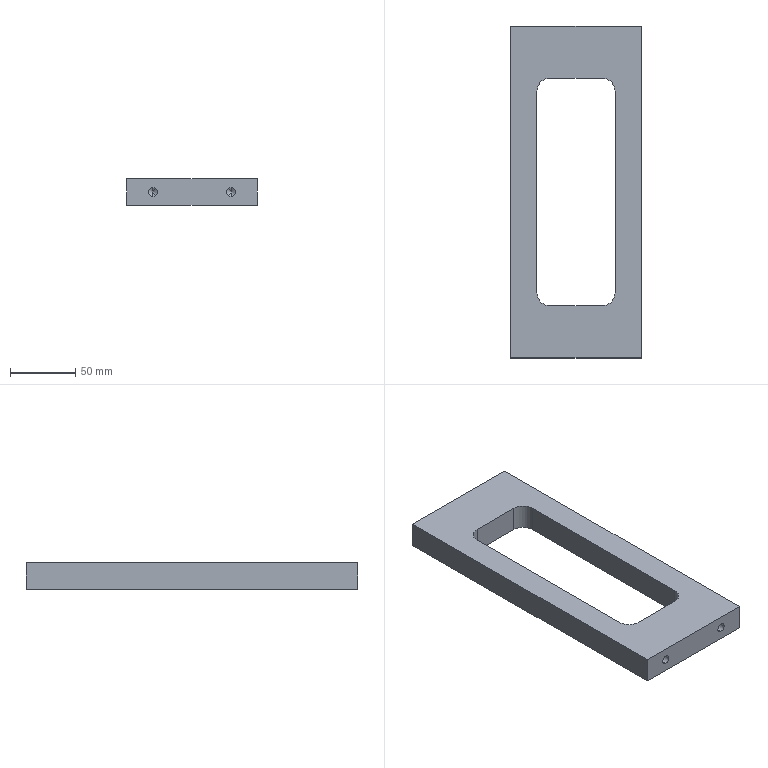Part | SolidWorks | features BaseBody 1 | 1 solid | 22 faces | box 100 x 255 x 20 mm | volume 300051 mm3 | plane 10 | cylinder 8 | cone 4 | commonest cylinder face diameters 6.8 x4 20 x4
STEP:
#1=CARTESIAN_POINT('',(-30.,-105.25,3.4));
#2=VERTEX_POINT('',#1);
#3=CARTESIAN_POINT('',(-30.,-105.25,-3.4));
#4=VERTEX_POINT('',#3);
#5=CARTESIAN_POINT('',(-30.,-105.25,0.));
#6=DIRECTION('',(0.,-1.,0.));
#7=DIRECTION('',(0.,0.,-1.));
#8=AXIS2_PLACEMENT_3D('',#5,#6,#7);
#9=CIRCLE('',#8,3.4);
#10=EDGE_CURVE('',#2,#4,#9,.T.);
#11=ORIENTED_EDGE('',*,*,#10,.F.);
#12=CARTESIAN_POINT('',(-30.,-127.5,3.4));
#13=VERTEX_POINT('',#12);
#14=CARTESIAN_POINT('',(-30.,-127.5,3.4));
#15=DIRECTION('',(0.,-1.,0.));
#16=VECTOR('',#15,1000.);
#17=LINE('',#14,#16);
#18=EDGE_CURVE('',#2,#13,#17,.T.);
#19=ORIENTED_EDGE('',*,*,#18,.T.);
#20=CARTESIAN_POINT('',(-30.,-127.5,-3.4));
#21=VERTEX_POINT('',#20);
#22=CARTESIAN_POINT('',(-30.,-127.5,0.));
#23=DIRECTION('',(0.,-1.,0.));
#24=DIRECTION('',(0.,0.,-1.));
#25=AXIS2_PLACEMENT_3D('',#22,#23,#24);
#26=CIRCLE('',#25,3.4);
#27=EDGE_CURVE('',#13,#21,#26,.T.);
#28=ORIENTED_EDGE('',*,*,#27,.T.);
#29=CARTESIAN_POINT('',(-30.,-127.5,-3.4));
#30=DIRECTION('',(0.,-1.,0.));
#31=VECTOR('',#30,1000.);
#32=LINE('',#29,#31);
#33=EDGE_CURVE('',#4,#21,#32,.T.);
#34=ORIENTED_EDGE('',*,*,#33,.F.);
#35=EDGE_LOOP('',(#11,#19,#28,#34));
#36=FACE_OUTER_BOUND('',#35,.T.);
#37=CARTESIAN_POINT('',(-30.,-127.5,0.));
#38=DIRECTION('',(0.,-1.,0.));
#39=DIRECTION('',(0.,0.,-1.));
#40=AXIS2_PLACEMENT_3D('',#37,#38,#39);
#41=CYLINDRICAL_SURFACE('',#40,3.4);
#42=ADVANCED_FACE('',(#36),#41,.F.);
#43=CARTESIAN_POINT('',(-30.,-103.207,0.));
#44=VERTEX_POINT('',#43);
#45=CARTESIAN_POINT('',(-30.,-105.25,-3.4));
#46=DIRECTION('',(0.,-0.515,-0.8572));
#47=VECTOR('',#46,1000.);
#48=LINE('',#45,#47);
#49=EDGE_CURVE('',#44,#4,#48,.T.);
#50=ORIENTED_EDGE('',*,*,#49,.F.);
#51=CARTESIAN_POINT('',(-30.,-105.25,3.4));
#52=DIRECTION('',(0.,-0.515,0.8572));
#53=VECTOR('',#52,1000.);
#54=LINE('',#51,#53);
#55=EDGE_CURVE('',#44,#2,#54,.T.);
#56=ORIENTED_EDGE('',*,*,#55,.T.);
#57=ORIENTED_EDGE('',*,*,#10,.T.);
#58=EDGE_LOOP('',(#50,#56,#57));
#59=FACE_OUTER_BOUND('',#58,.T.);
#60=CARTESIAN_POINT('',(-30.,-105.25,0.));
#61=DIRECTION('',(0.,-1.,0.));
#62=DIRECTION('',(0.,0.,-1.));
#63=AXIS2_PLACEMENT_3D('',#60,#61,#62);
#64=CONICAL_SURFACE('',#63,3.4,1.03);
#65=ADVANCED_FACE('',(#59),#64,.F.);
#66=CARTESIAN_POINT('',(30.,-105.25,3.4));
#67=VERTEX_POINT('',#66);
#68=CARTESIAN_POINT('',(30.,-105.25,-3.4));
#69=VERTEX_POINT('',#68);
#70=CARTESIAN_POINT('',(30.,-105.25,0.));
#71=DIRECTION('',(0.,-1.,0.));
#72=DIRECTION('',(0.,0.,-1.));
#73=AXIS2_PLACEMENT_3D('',#70,#71,#72);
#74=CIRCLE('',#73,3.4);
#75=EDGE_CURVE('',#67,#69,#74,.T.);
#76=ORIENTED_EDGE('',*,*,#75,.F.);
#77=CARTESIAN_POINT('',(30.,-127.5,3.4));
#78=VERTEX_POINT('',#77);
#79=CARTESIAN_POINT('',(30.,-127.5,3.4));
#80=DIRECTION('',(0.,-1.,0.));
#81=VECTOR('',#80,1000.);
#82=LINE('',#79,#81);
#83=EDGE_CURVE('',#67,#78,#82,.T.);
#84=ORIENTED_EDGE('',*,*,#83,.T.);
#85=CARTESIAN_POINT('',(30.,-127.5,-3.4));
#86=VERTEX_POINT('',#85);
#87=CARTESIAN_POINT('',(30.,-127.5,0.));
#88=DIRECTION('',(0.,-1.,0.));
#89=DIRECTION('',(0.,0.,-1.));
#90=AXIS2_PLACEMENT_3D('',#87,#88,#89);
#91=CIRCLE('',#90,3.4);
#92=EDGE_CURVE('',#78,#86,#91,.T.);
#93=ORIENTED_EDGE('',*,*,#92,.T.);
#94=CARTESIAN_POINT('',(30.,-127.5,-3.4));
#95=DIRECTION('',(0.,-1.,0.));
#96=VECTOR('',#95,1000.);
#97=LINE('',#94,#96);
#98=EDGE_CURVE('',#69,#86,#97,.T.);
#99=ORIENTED_EDGE('',*,*,#98,.F.);
#100=EDGE_LOOP('',(#76,#84,#93,#99));
#101=FACE_OUTER_BOUND('',#100,.T.);
#102=CARTESIAN_POINT('',(30.,-127.5,0.));
#103=DIRECTION('',(0.,-1.,0.));
#104=DIRECTION('',(0.,0.,-1.));
#105=AXIS2_PLACEMENT_3D('',#102,#103,#104);
#106=CYLINDRICAL_SURFACE('',#105,3.4);
#107=ADVANCED_FACE('',(#101),#106,.F.);
#108=CARTESIAN_POINT('',(30.,-103.207,0.));
#109=VERTEX_POINT('',#108);
#110=CARTESIAN_POINT('',(30.,-105.25,-3.4));
#111=DIRECTION('',(0.,-0.515,-0.8572));
#112=VECTOR('',#111,1000.);
#113=LINE('',#110,#112);
#114=EDGE_CURVE('',#109,#69,#113,.T.);
#115=ORIENTED_EDGE('',*,*,#114,.F.);
#116=CARTESIAN_POINT('',(30.,-105.25,3.4));
#117=DIRECTION('',(0.,-0.515,0.8572));
#118=VECTOR('',#117,1000.);
#119=LINE('',#116,#118);
#120=EDGE_CURVE('',#109,#67,#119,.T.);
#121=ORIENTED_EDGE('',*,*,#120,.T.);
#122=ORIENTED_EDGE('',*,*,#75,.T.);
#123=EDGE_LOOP('',(#115,#121,#122));
#124=FACE_OUTER_BOUND('',#123,.T.);
#125=CARTESIAN_POINT('',(30.,-105.25,0.));
#126=DIRECTION('',(0.,-1.,0.));
#127=DIRECTION('',(0.,0.,-1.));
#128=AXIS2_PLACEMENT_3D('',#125,#126,#127);
#129=CONICAL_SURFACE('',#128,3.4,1.03);
#130=ADVANCED_FACE('',(#124),#129,.F.);
#131=CARTESIAN_POINT('',(-50.,127.5,-10.));
#132=VERTEX_POINT('',#131);
#133=CARTESIAN_POINT('',(-50.,-127.5,-10.));
#134=VERTEX_POINT('',#133);
#135=CARTESIAN_POINT('',(-50.,127.5,-10.));
#136=DIRECTION('',(0.,-1.,0.));
#137=VECTOR('',#136,1000.);
#138=LINE('',#135,#137);
#139=EDGE_CURVE('',#132,#134,#138,.T.);
#140=ORIENTED_EDGE('',*,*,#139,.T.);
#141=CARTESIAN_POINT('',(-50.,-127.5,10.));
#142=VERTEX_POINT('',#141);
#143=CARTESIAN_POINT('',(-50.,-127.5,10.));
#144=DIRECTION('',(0.,0.,-1.));
#145=VECTOR('',#144,1000.);
#146=LINE('',#143,#145);
#147=EDGE_CURVE('',#142,#134,#146,.T.);
#148=ORIENTED_EDGE('',*,*,#147,.F.);
#149=CARTESIAN_POINT('',(-50.,127.5,10.));
#150=VERTEX_POINT('',#149);
#151=CARTESIAN_POINT('',(-50.,127.5,10.));
#152=DIRECTION('',(0.,-1.,0.));
#153=VECTOR('',#152,1000.);
#154=LINE('',#151,#153);
#155=EDGE_CURVE('',#150,#142,#154,.T.);
#156=ORIENTED_EDGE('',*,*,#155,.F.);
#157=CARTESIAN_POINT('',(-50.,127.5,10.));
#158=DIRECTION('',(0.,0.,-1.));
#159=VECTOR('',#158,1000.);
#160=LINE('',#157,#159);
#161=EDGE_CURVE('',#150,#132,#160,.T.);
#162=ORIENTED_EDGE('',*,*,#161,.T.);
#163=EDGE_LOOP('',(#140,#148,#156,#162));
#164=FACE_OUTER_BOUND('',#163,.T.);
#165=CARTESIAN_POINT('',(-50.,127.5,10.));
#166=DIRECTION('',(1.,0.,0.));
#167=DIRECTION('',(0.,1.,0.));
#168=AXIS2_PLACEMENT_3D('',#165,#166,#167);
#169=PLANE('',#168);
#170=ADVANCED_FACE('',(#164),#169,.F.);
#171=CARTESIAN_POINT('',(-30.,-127.5,0.));
#172=DIRECTION('',(0.,-1.,0.));
#173=DIRECTION('',(0.,0.,-1.));
#174=AXIS2_PLACEMENT_3D('',#171,#172,#173);
#175=CIRCLE('',#174,3.4);
#176=EDGE_CURVE('',#21,#13,#175,.T.);
#177=ORIENTED_EDGE('',*,*,#176,.F.);
#178=ORIENTED_EDGE('',*,*,#27,.F.);
#179=EDGE_LOOP('',(#177,#178));
#180=FACE_BOUND('',#179,.T.);
#181=CARTESIAN_POINT('',(30.,-127.5,0.));
#182=DIRECTION('',(0.,-1.,0.));
#183=DIRECTION('',(0.,0.,-1.));
#184=AXIS2_PLACEMENT_3D('',#181,#182,#183);
#185=CIRCLE('',#184,3.4);
#186=EDGE_CURVE('',#86,#78,#185,.T.);
#187=ORIENTED_EDGE('',*,*,#186,.F.);
#188=ORIENTED_EDGE('',*,*,#92,.F.);
#189=EDGE_LOOP('',(#187,#188));
#190=FACE_BOUND('',#189,.T.);
#191=CARTESIAN_POINT('',(50.,-127.5,-10.));
#192=VERTEX_POINT('',#191);
#193=CARTESIAN_POINT('',(50.,-127.5,-10.));
#194=DIRECTION('',(1.,0.,0.));
#195=VECTOR('',#194,1000.);
#196=LINE('',#193,#195);
#197=EDGE_CURVE('',#134,#192,#196,.T.);
#198=ORIENTED_EDGE('',*,*,#197,.T.);
#199=CARTESIAN_POINT('',(50.,-127.5,10.));
#200=VERTEX_POINT('',#199);
#201=CARTESIAN_POINT('',(50.,-127.5,10.));
#202=DIRECTION('',(0.,0.,-1.));
#203=VECTOR('',#202,1000.);
#204=LINE('',#201,#203);
#205=EDGE_CURVE('',#200,#192,#204,.T.);
#206=ORIENTED_EDGE('',*,*,#205,.F.);
#207=CARTESIAN_POINT('',(50.,-127.5,10.));
#208=DIRECTION('',(1.,0.,0.));
#209=VECTOR('',#208,1000.);
#210=LINE('',#207,#209);
#211=EDGE_CURVE('',#142,#200,#210,.T.);
#212=ORIENTED_EDGE('',*,*,#211,.F.);
#213=ORIENTED_EDGE('',*,*,#147,.T.);
#214=EDGE_LOOP('',(#198,#206,#212,#213));
#215=FACE_OUTER_BOUND('',#214,.T.);
#216=CARTESIAN_POINT('',(50.,-127.5,10.));
#217=DIRECTION('',(0.,1.,0.));
#218=DIRECTION('',(0.,0.,1.));
#219=AXIS2_PLACEMENT_3D('',#216,#217,#218);
#220=PLANE('',#219);
#221=ADVANCED_FACE('',(#180,#190,#215),#220,.F.);
#222=CARTESIAN_POINT('',(50.,127.5,-10.));
#223=VERTEX_POINT('',#222);
#224=CARTESIAN_POINT('',(50.,127.5,-10.));
#225=DIRECTION('',(0.,1.,0.));
#226=VECTOR('',#225,1000.);
#227=LINE('',#224,#226);
#228=EDGE_CURVE('',#192,#223,#227,.T.);
#229=ORIENTED_EDGE('',*,*,#228,.T.);
#230=CARTESIAN_POINT('',(50.,127.5,10.));
#231=VERTEX_POINT('',#230);
#232=CARTESIAN_POINT('',(50.,127.5,10.));
#233=DIRECTION('',(0.,0.,-1.));
#234=VECTOR('',#233,1000.);
#235=LINE('',#232,#234);
#236=EDGE_CURVE('',#231,#223,#235,.T.);
#237=ORIENTED_EDGE('',*,*,#236,.F.);
#238=CARTESIAN_POINT('',(50.,127.5,10.));
#239=DIRECTION('',(0.,1.,0.));
#240=VECTOR('',#239,1000.);
#241=LINE('',#238,#240);
#242=EDGE_CURVE('',#200,#231,#241,.T.);
#243=ORIENTED_EDGE('',*,*,#242,.F.);
#244=ORIENTED_EDGE('',*,*,#205,.T.);
#245=EDGE_LOOP('',(#229,#237,#243,#244));
#246=FACE_OUTER_BOUND('',#245,.T.);
#247=CARTESIAN_POINT('',(50.,127.5,10.));
#248=DIRECTION('',(-1.,0.,0.));
#249=DIRECTION('',(0.,-1.,0.));
#250=AXIS2_PLACEMENT_3D('',#247,#248,#249);
#251=PLANE('',#250);
#252=ADVANCED_FACE('',(#246),#251,.F.);
#253=CARTESIAN_POINT('',(50.,127.5,-10.));
#254=DIRECTION('',(-1.,0.,0.));
#255=VECTOR('',#254,1000.);
#256=LINE('',#253,#255);
#257=EDGE_CURVE('',#223,#132,#256,.T.);
#258=ORIENTED_EDGE('',*,*,#257,.T.);
#259=ORIENTED_EDGE('',*,*,#161,.F.);
#260=CARTESIAN_POINT('',(50.,127.5,10.));
#261=DIRECTION('',(-1.,0.,0.));
#262=VECTOR('',#261,1000.);
#263=LINE('',#260,#262);
#264=EDGE_CURVE('',#231,#150,#263,.T.);
#265=ORIENTED_EDGE('',*,*,#264,.F.);
#266=ORIENTED_EDGE('',*,*,#236,.T.);
#267=EDGE_LOOP('',(#258,#259,#265,#266));
#268=FACE_OUTER_BOUND('',#267,.T.);
#269=CARTESIAN_POINT('',(50.,127.5,10.));
#270=DIRECTION('',(0.,-1.,0.));
#271=DIRECTION('',(1.,0.,0.));
#272=AXIS2_PLACEMENT_3D('',#269,#270,#271);
#273=PLANE('',#272);
#274=ADVANCED_FACE('',(#268),#273,.F.);
#275=CARTESIAN_POINT('',(30.,77.5,10.));
#276=VERTEX_POINT('',#275);
#277=CARTESIAN_POINT('',(30.,-77.5,10.));
#278=VERTEX_POINT('',#277);
#279=CARTESIAN_POINT('',(30.,77.5,10.));
#280=DIRECTION('',(0.,-1.,0.));
#281=VECTOR('',#280,1000.);
#282=LINE('',#279,#281);
#283=EDGE_CURVE('',#276,#278,#282,.T.);
#284=ORIENTED_EDGE('',*,*,#283,.T.);
#285=CARTESIAN_POINT('',(20.,-87.5,10.));
#286=VERTEX_POINT('',#285);
#287=CARTESIAN_POINT('',(20.,-77.5,10.));
#288=DIRECTION('',(0.,0.,-1.));
#289=DIRECTION('',(-1.,0.,0.));
#290=AXIS2_PLACEMENT_3D('',#287,#288,#289);
#291=CIRCLE('',#290,10.);
#292=EDGE_CURVE('',#278,#286,#291,.T.);
#293=ORIENTED_EDGE('',*,*,#292,.T.);
#294=CARTESIAN_POINT('',(-20.,-87.5,10.));
#295=VERTEX_POINT('',#294);
#296=CARTESIAN_POINT('',(-20.,-87.5,10.));
#297=DIRECTION('',(-1.,0.,0.));
#298=VECTOR('',#297,1000.);
#299=LINE('',#296,#298);
#300=EDGE_CURVE('',#286,#295,#299,.T.);
#301=ORIENTED_EDGE('',*,*,#300,.T.);
#302=CARTESIAN_POINT('',(-30.,-77.5,10.));
#303=VERTEX_POINT('',#302);
#304=CARTESIAN_POINT('',(-20.,-77.5,10.));
#305=DIRECTION('',(0.,0.,-1.));
#306=DIRECTION('',(-1.,0.,0.));
#307=AXIS2_PLACEMENT_3D('',#304,#305,#306);
#308=CIRCLE('',#307,10.);
#309=EDGE_CURVE('',#295,#303,#308,.T.);
#310=ORIENTED_EDGE('',*,*,#309,.T.);
#311=CARTESIAN_POINT('',(-30.,77.5,10.));
#312=VERTEX_POINT('',#311);
#313=CARTESIAN_POINT('',(-30.,77.5,10.));
#314=DIRECTION('',(0.,1.,0.));
#315=VECTOR('',#314,1000.);
#316=LINE('',#313,#315);
#317=EDGE_CURVE('',#303,#312,#316,.T.);
#318=ORIENTED_EDGE('',*,*,#317,.T.);
#319=CARTESIAN_POINT('',(-20.,87.5,10.));
#320=VERTEX_POINT('',#319);
#321=CARTESIAN_POINT('',(-20.,77.5,10.));
#322=DIRECTION('',(0.,0.,-1.));
#323=DIRECTION('',(1.,0.,0.));
#324=AXIS2_PLACEMENT_3D('',#321,#322,#323);
#325=CIRCLE('',#324,10.);
#326=EDGE_CURVE('',#312,#320,#325,.T.);
#327=ORIENTED_EDGE('',*,*,#326,.T.);
#328=CARTESIAN_POINT('',(20.,87.5,10.));
#329=VERTEX_POINT('',#328);
#330=CARTESIAN_POINT('',(-20.,87.5,10.));
#331=DIRECTION('',(1.,0.,0.));
#332=VECTOR('',#331,1000.);
#333=LINE('',#330,#332);
#334=EDGE_CURVE('',#320,#329,#333,.T.);
#335=ORIENTED_EDGE('',*,*,#334,.T.);
#336=CARTESIAN_POINT('',(20.,77.5,10.));
#337=DIRECTION('',(0.,0.,-1.));
#338=DIRECTION('',(1.,0.,0.));
#339=AXIS2_PLACEMENT_3D('',#336,#337,#338);
#340=CIRCLE('',#339,10.);
#341=EDGE_CURVE('',#329,#276,#340,.T.);
#342=ORIENTED_EDGE('',*,*,#341,.T.);
#343=EDGE_LOOP('',(#284,#293,#301,#310,#318,#327,#335,#342));
#344=FACE_BOUND('',#343,.T.);
#345=ORIENTED_EDGE('',*,*,#155,.T.);
#346=ORIENTED_EDGE('',*,*,#211,.T.);
#347=ORIENTED_EDGE('',*,*,#242,.T.);
#348=ORIENTED_EDGE('',*,*,#264,.T.);
#349=EDGE_LOOP('',(#345,#346,#347,#348));
#350=FACE_OUTER_BOUND('',#349,.T.);
#351=CARTESIAN_POINT('',(-50.,-127.5,10.));
#352=DIRECTION('',(0.,0.,-1.));
#353=DIRECTION('',(-1.,0.,0.));
#354=AXIS2_PLACEMENT_3D('',#351,#352,#353);
#355=PLANE('',#354);
#356=ADVANCED_FACE('',(#344,#350),#355,.F.);
#357=CARTESIAN_POINT('',(30.,-77.5,-10.));
#358=VERTEX_POINT('',#357);
#359=CARTESIAN_POINT('',(20.,-87.5,-10.));
#360=VERTEX_POINT('',#359);
#361=CARTESIAN_POINT('',(20.,-77.5,-10.));
#362=DIRECTION('',(0.,0.,-1.));
#363=DIRECTION('',(-1.,0.,0.));
#364=AXIS2_PLACEMENT_3D('',#361,#362,#363);
#365=CIRCLE('',#364,10.);
#366=EDGE_CURVE('',#358,#360,#365,.T.);
#367=ORIENTED_EDGE('',*,*,#366,.F.);
#368=CARTESIAN_POINT('',(30.,77.5,-10.));
#369=VERTEX_POINT('',#368);
#370=CARTESIAN_POINT('',(30.,77.5,-10.));
#371=DIRECTION('',(0.,-1.,0.));
#372=VECTOR('',#371,1000.);
#373=LINE('',#370,#372);
#374=EDGE_CURVE('',#369,#358,#373,.T.);
#375=ORIENTED_EDGE('',*,*,#374,.F.);
#376=CARTESIAN_POINT('',(20.,87.5,-10.));
#377=VERTEX_POINT('',#376);
#378=CARTESIAN_POINT('',(20.,77.5,-10.));
#379=DIRECTION('',(0.,0.,-1.));
#380=DIRECTION('',(1.,0.,0.));
#381=AXIS2_PLACEMENT_3D('',#378,#379,#380);
#382=CIRCLE('',#381,10.);
#383=EDGE_CURVE('',#377,#369,#382,.T.);
#384=ORIENTED_EDGE('',*,*,#383,.F.);
#385=CARTESIAN_POINT('',(-20.,87.5,-10.));
#386=VERTEX_POINT('',#385);
#387=CARTESIAN_POINT('',(-20.,87.5,-10.));
#388=DIRECTION('',(1.,0.,0.));
#389=VECTOR('',#388,1000.);
#390=LINE('',#387,#389);
#391=EDGE_CURVE('',#386,#377,#390,.T.);
#392=ORIENTED_EDGE('',*,*,#391,.F.);
#393=CARTESIAN_POINT('',(-30.,77.5,-10.));
#394=VERTEX_POINT('',#393);
#395=CARTESIAN_POINT('',(-20.,77.5,-10.));
#396=DIRECTION('',(0.,0.,-1.));
#397=DIRECTION('',(1.,0.,0.));
#398=AXIS2_PLACEMENT_3D('',#395,#396,#397);
#399=CIRCLE('',#398,10.);
#400=EDGE_CURVE('',#394,#386,#399,.T.);
#401=ORIENTED_EDGE('',*,*,#400,.F.);
#402=CARTESIAN_POINT('',(-30.,-77.5,-10.));
#403=VERTEX_POINT('',#402);
#404=CARTESIAN_POINT('',(-30.,77.5,-10.));
#405=DIRECTION('',(0.,1.,0.));
#406=VECTOR('',#405,1000.);
#407=LINE('',#404,#406);
#408=EDGE_CURVE('',#403,#394,#407,.T.);
#409=ORIENTED_EDGE('',*,*,#408,.F.);
#410=CARTESIAN_POINT('',(-20.,-87.5,-10.));
#411=VERTEX_POINT('',#410);
#412=CARTESIAN_POINT('',(-20.,-77.5,-10.));
#413=DIRECTION('',(0.,0.,-1.));
#414=DIRECTION('',(-1.,0.,0.));
#415=AXIS2_PLACEMENT_3D('',#412,#413,#414);
#416=CIRCLE('',#415,10.);
#417=EDGE_CURVE('',#411,#403,#416,.T.);
#418=ORIENTED_EDGE('',*,*,#417,.F.);
#419=CARTESIAN_POINT('',(-20.,-87.5,-10.));
#420=DIRECTION('',(-1.,0.,0.));
#421=VECTOR('',#420,1000.);
#422=LINE('',#419,#421);
#423=EDGE_CURVE('',#360,#411,#422,.T.);
#424=ORIENTED_EDGE('',*,*,#423,.F.);
#425=EDGE_LOOP('',(#367,#375,#384,#392,#401,#409,#418,#424));
#426=FACE_BOUND('',#425,.T.);
#427=ORIENTED_EDGE('',*,*,#139,.F.);
#428=ORIENTED_EDGE('',*,*,#257,.F.);
#429=ORIENTED_EDGE('',*,*,#228,.F.);
#430=ORIENTED_EDGE('',*,*,#197,.F.);
#431=EDGE_LOOP('',(#427,#428,#429,#430));
#432=FACE_OUTER_BOUND('',#431,.T.);
#433=CARTESIAN_POINT('',(-50.,-127.5,-10.));
#434=DIRECTION('',(0.,0.,-1.));
#435=DIRECTION('',(-1.,0.,0.));
#436=AXIS2_PLACEMENT_3D('',#433,#434,#435);
#437=PLANE('',#436);
#438=ADVANCED_FACE('',(#426,#432),#437,.T.);
#439=ORIENTED_EDGE('',*,*,#366,.T.);
#440=CARTESIAN_POINT('',(20.,-87.5,10.));
#441=DIRECTION('',(0.,0.,-1.));
#442=VECTOR('',#441,1000.);
#443=LINE('',#440,#442);
#444=EDGE_CURVE('',#286,#360,#443,.T.);
#445=ORIENTED_EDGE('',*,*,#444,.F.);
#446=ORIENTED_EDGE('',*,*,#292,.F.);
#447=CARTESIAN_POINT('',(30.,-77.5,10.));
#448=DIRECTION('',(0.,0.,-1.));
#449=VECTOR('',#448,1000.);
#450=LINE('',#447,#449);
#451=EDGE_CURVE('',#278,#358,#450,.T.);
#452=ORIENTED_EDGE('',*,*,#451,.T.);
#453=EDGE_LOOP('',(#439,#445,#446,#452));
#454=FACE_OUTER_BOUND('',#453,.T.);
#455=CARTESIAN_POINT('',(20.,-77.5,10.));
#456=DIRECTION('',(0.,0.,-1.));
#457=DIRECTION('',(-1.,0.,0.));
#458=AXIS2_PLACEMENT_3D('',#455,#456,#457);
#459=CYLINDRICAL_SURFACE('',#458,10.);
#460=ADVANCED_FACE('',(#454),#459,.F.);
#461=ORIENTED_EDGE('',*,*,#374,.T.);
#462=ORIENTED_EDGE('',*,*,#451,.F.);
#463=ORIENTED_EDGE('',*,*,#283,.F.);
#464=CARTESIAN_POINT('',(30.,77.5,10.));
#465=DIRECTION('',(0.,0.,-1.));
#466=VECTOR('',#465,1000.);
#467=LINE('',#464,#466);
#468=EDGE_CURVE('',#276,#369,#467,.T.);
#469=ORIENTED_EDGE('',*,*,#468,.T.);
#470=EDGE_LOOP('',(#461,#462,#463,#469));
#471=FACE_OUTER_BOUND('',#470,.T.);
#472=CARTESIAN_POINT('',(30.,77.5,10.));
#473=DIRECTION('',(1.,0.,0.));
#474=DIRECTION('',(0.,1.,0.));
#475=AXIS2_PLACEMENT_3D('',#472,#473,#474);
#476=PLANE('',#475);
#477=ADVANCED_FACE('',(#471),#476,.F.);
#478=ORIENTED_EDGE('',*,*,#383,.T.);
#479=ORIENTED_EDGE('',*,*,#468,.F.);
#480=ORIENTED_EDGE('',*,*,#341,.F.);
#481=CARTESIAN_POINT('',(20.,87.5,10.));
#482=DIRECTION('',(0.,0.,-1.));
#483=VECTOR('',#482,1000.);
#484=LINE('',#481,#483);
#485=EDGE_CURVE('',#329,#377,#484,.T.);
#486=ORIENTED_EDGE('',*,*,#485,.T.);
#487=EDGE_LOOP('',(#478,#479,#480,#486));
#488=FACE_OUTER_BOUND('',#487,.T.);
#489=CARTESIAN_POINT('',(20.,77.5,10.));
#490=DIRECTION('',(0.,0.,-1.));
#491=DIRECTION('',(-1.,0.,0.));
#492=AXIS2_PLACEMENT_3D('',#489,#490,#491);
#493=CYLINDRICAL_SURFACE('',#492,10.);
#494=ADVANCED_FACE('',(#488),#493,.F.);
#495=ORIENTED_EDGE('',*,*,#391,.T.);
#496=ORIENTED_EDGE('',*,*,#485,.F.);
#497=ORIENTED_EDGE('',*,*,#334,.F.);
#498=CARTESIAN_POINT('',(-20.,87.5,10.));
#499=DIRECTION('',(0.,0.,-1.));
#500=VECTOR('',#499,1000.);
#501=LINE('',#498,#500);
#502=EDGE_CURVE('',#320,#386,#501,.T.);
#503=ORIENTED_EDGE('',*,*,#502,.T.);
#504=EDGE_LOOP('',(#495,#496,#497,#503));
#505=FACE_OUTER_BOUND('',#504,.T.);
#506=CARTESIAN_POINT('',(-20.,87.5,10.));
#507=DIRECTION('',(0.,1.,0.));
#508=DIRECTION('',(-1.,0.,0.));
#509=AXIS2_PLACEMENT_3D('',#506,#507,#508);
#510=PLANE('',#509);
#511=ADVANCED_FACE('',(#505),#510,.F.);
#512=ORIENTED_EDGE('',*,*,#400,.T.);
#513=ORIENTED_EDGE('',*,*,#502,.F.);
#514=ORIENTED_EDGE('',*,*,#326,.F.);
#515=CARTESIAN_POINT('',(-30.,77.5,10.));
#516=DIRECTION('',(0.,0.,-1.));
#517=VECTOR('',#516,1000.);
#518=LINE('',#515,#517);
#519=EDGE_CURVE('',#312,#394,#518,.T.);
#520=ORIENTED_EDGE('',*,*,#519,.T.);
#521=EDGE_LOOP('',(#512,#513,#514,#520));
#522=FACE_OUTER_BOUND('',#521,.T.);
#523=CARTESIAN_POINT('',(-20.,77.5,10.));
#524=DIRECTION('',(0.,0.,-1.));
#525=DIRECTION('',(-1.,0.,0.));
#526=AXIS2_PLACEMENT_3D('',#523,#524,#525);
#527=CYLINDRICAL_SURFACE('',#526,10.);
#528=ADVANCED_FACE('',(#522),#527,.F.);
#529=ORIENTED_EDGE('',*,*,#408,.T.);
#530=ORIENTED_EDGE('',*,*,#519,.F.);
#531=ORIENTED_EDGE('',*,*,#317,.F.);
#532=CARTESIAN_POINT('',(-30.,-77.5,10.));
#533=DIRECTION('',(0.,0.,-1.));
#534=VECTOR('',#533,1000.);
#535=LINE('',#532,#534);
#536=EDGE_CURVE('',#303,#403,#535,.T.);
#537=ORIENTED_EDGE('',*,*,#536,.T.);
#538=EDGE_LOOP('',(#529,#530,#531,#537));
#539=FACE_OUTER_BOUND('',#538,.T.);
#540=CARTESIAN_POINT('',(-30.,77.5,10.));
#541=DIRECTION('',(-1.,0.,0.));
#542=DIRECTION('',(0.,0.,1.));
#543=AXIS2_PLACEMENT_3D('',#540,#541,#542);
#544=PLANE('',#543);
#545=ADVANCED_FACE('',(#539),#544,.F.);
#546=ORIENTED_EDGE('',*,*,#417,.T.);
#547=ORIENTED_EDGE('',*,*,#536,.F.);
#548=ORIENTED_EDGE('',*,*,#309,.F.);
#549=CARTESIAN_POINT('',(-20.,-87.5,10.));
#550=DIRECTION('',(0.,0.,-1.));
#551=VECTOR('',#550,1000.);
#552=LINE('',#549,#551);
#553=EDGE_CURVE('',#295,#411,#552,.T.);
#554=ORIENTED_EDGE('',*,*,#553,.T.);
#555=EDGE_LOOP('',(#546,#547,#548,#554));
#556=FACE_OUTER_BOUND('',#555,.T.);
#557=CARTESIAN_POINT('',(-20.,-77.5,10.));
#558=DIRECTION('',(0.,0.,-1.));
#559=DIRECTION('',(-1.,0.,0.));
#560=AXIS2_PLACEMENT_3D('',#557,#558,#559);
#561=CYLINDRICAL_SURFACE('',#560,10.);
#562=ADVANCED_FACE('',(#556),#561,.F.);
#563=ORIENTED_EDGE('',*,*,#423,.T.);
#564=ORIENTED_EDGE('',*,*,#553,.F.);
#565=ORIENTED_EDGE('',*,*,#300,.F.);
#566=ORIENTED_EDGE('',*,*,#444,.T.);
#567=EDGE_LOOP('',(#563,#564,#565,#566));
#568=FACE_OUTER_BOUND('',#567,.T.);
#569=CARTESIAN_POINT('',(-20.,-87.5,10.));
#570=DIRECTION('',(0.,-1.,0.));
#571=DIRECTION('',(0.,0.,-1.));
#572=AXIS2_PLACEMENT_3D('',#569,#570,#571);
#573=PLANE('',#572);
#574=ADVANCED_FACE('',(#568),#573,.F.);
#575=ORIENTED_EDGE('',*,*,#120,.F.);
#576=ORIENTED_EDGE('',*,*,#114,.T.);
#577=CARTESIAN_POINT('',(30.,-105.25,0.));
#578=DIRECTION('',(0.,-1.,0.));
#579=DIRECTION('',(0.,0.,-1.));
#580=AXIS2_PLACEMENT_3D('',#577,#578,#579);
#581=CIRCLE('',#580,3.4);
#582=EDGE_CURVE('',#69,#67,#581,.T.);
#583=ORIENTED_EDGE('',*,*,#582,.T.);
#584=EDGE_LOOP('',(#575,#576,#583));
#585=FACE_OUTER_BOUND('',#584,.T.);
#586=CARTESIAN_POINT('',(30.,-105.25,0.));
#587=DIRECTION('',(0.,-1.,0.));
#588=DIRECTION('',(0.,0.,-1.));
#589=AXIS2_PLACEMENT_3D('',#586,#587,#588);
#590=CONICAL_SURFACE('',#589,3.4,1.03);
#591=ADVANCED_FACE('',(#585),#590,.F.);
#592=ORIENTED_EDGE('',*,*,#83,.F.);
#593=ORIENTED_EDGE('',*,*,#582,.F.);
#594=ORIENTED_EDGE('',*,*,#98,.T.);
#595=ORIENTED_EDGE('',*,*,#186,.T.);
#596=EDGE_LOOP('',(#592,#593,#594,#595));
#597=FACE_OUTER_BOUND('',#596,.T.);
#598=CARTESIAN_POINT('',(30.,-127.5,0.));
#599=DIRECTION('',(0.,-1.,0.));
#600=DIRECTION('',(0.,0.,-1.));
#601=AXIS2_PLACEMENT_3D('',#598,#599,#600);
#602=CYLINDRICAL_SURFACE('',#601,3.4);
#603=ADVANCED_FACE('',(#597),#602,.F.);
#604=ORIENTED_EDGE('',*,*,#55,.F.);
#605=ORIENTED_EDGE('',*,*,#49,.T.);
#606=CARTESIAN_POINT('',(-30.,-105.25,0.));
#607=DIRECTION('',(0.,-1.,0.));
#608=DIRECTION('',(0.,0.,-1.));
#609=AXIS2_PLACEMENT_3D('',#606,#607,#608);
#610=CIRCLE('',#609,3.4);
#611=EDGE_CURVE('',#4,#2,#610,.T.);
#612=ORIENTED_EDGE('',*,*,#611,.T.);
#613=EDGE_LOOP('',(#604,#605,#612));
#614=FACE_OUTER_BOUND('',#613,.T.);
#615=CARTESIAN_POINT('',(-30.,-105.25,0.));
#616=DIRECTION('',(0.,-1.,0.));
#617=DIRECTION('',(0.,0.,-1.));
#618=AXIS2_PLACEMENT_3D('',#615,#616,#617);
#619=CONICAL_SURFACE('',#618,3.4,1.03);
#620=ADVANCED_FACE('',(#614),#619,.F.);
#621=ORIENTED_EDGE('',*,*,#18,.F.);
#622=ORIENTED_EDGE('',*,*,#611,.F.);
#623=ORIENTED_EDGE('',*,*,#33,.T.);
#624=ORIENTED_EDGE('',*,*,#176,.T.);
#625=EDGE_LOOP('',(#621,#622,#623,#624));
#626=FACE_OUTER_BOUND('',#625,.T.);
#627=CARTESIAN_POINT('',(-30.,-127.5,0.));
#628=DIRECTION('',(0.,-1.,0.));
#629=DIRECTION('',(0.,0.,-1.));
#630=AXIS2_PLACEMENT_3D('',#627,#628,#629);
#631=CYLINDRICAL_SURFACE('',#630,3.4);
#632=ADVANCED_FACE('',(#626),#631,.F.);
#633=CLOSED_SHELL('',(#42,#65,#107,#130,#170,#221,#252,#274,#356,#438,#460,#477,#494,#511,#528,#545,#562,#574,#591,#603,#620,#632));
#634=MANIFOLD_SOLID_BREP('',#633);
#635=CARTESIAN_POINT('',(0.,0.,0.));
#636=DIRECTION('',(0.,0.,1.));
#637=DIRECTION('',(1.,0.,0.));
#638=AXIS2_PLACEMENT_3D('',#635,#636,#637);
#639=(LENGTH_UNIT()NAMED_UNIT(*)SI_UNIT(.MILLI.,.METRE.));
#640=UNCERTAINTY_MEASURE_WITH_UNIT(LENGTH_MEASURE(0.00001),#639,'','');
#641=(NAMED_UNIT(*)PLANE_ANGLE_UNIT()SI_UNIT($,.RADIAN.));
#642=(NAMED_UNIT(*)SI_UNIT($,.STERADIAN.)SOLID_ANGLE_UNIT());
#643=(GEOMETRIC_REPRESENTATION_CONTEXT(3)GLOBAL_UNCERTAINTY_ASSIGNED_CONTEXT((#640))GLOBAL_UNIT_ASSIGNED_CONTEXT((#639,#641,#642))REPRESENTATION_CONTEXT('',''));
#644=ADVANCED_BREP_SHAPE_REPRESENTATION('',(#634,#638),#643);